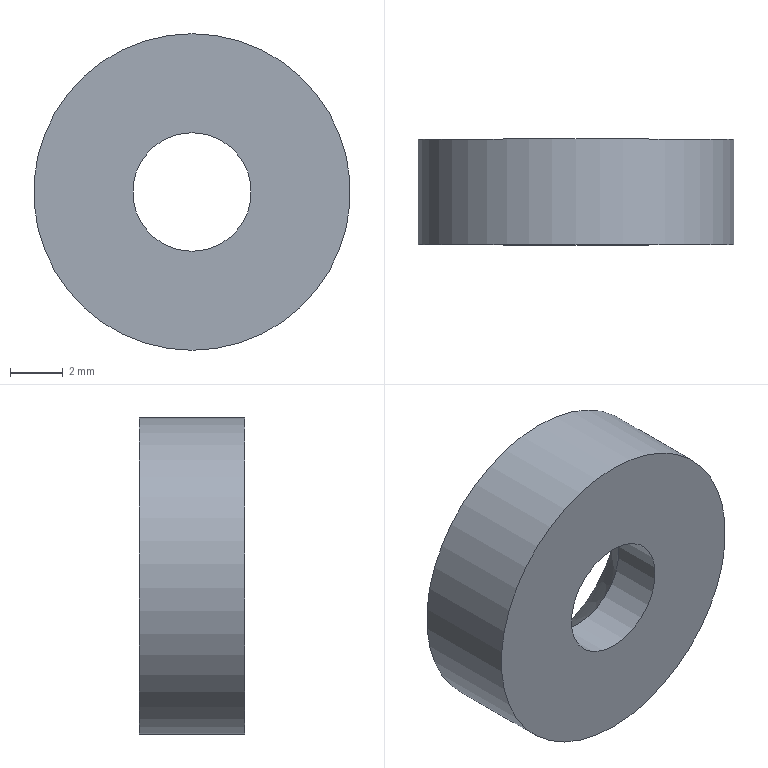Part | STEP file | Strong magnet | 1 solid | 5 faces | box 12 x 4 x 12 mm | volume 350.045 mm3 | cylinder 2 | plane 2 | cone 1 | commonest cylinder face diameters 4.5 x1 12 x1
STEP:
#1=CARTESIAN_POINT('',(0.,4.,6.));
#2=VERTEX_POINT('',#1);
#3=CARTESIAN_POINT('',(0.,4.,0.));
#4=DIRECTION('',(0.,1.,0.));
#5=DIRECTION('',(0.,0.,1.));
#6=AXIS2_PLACEMENT_3D('',#3,#4,#5);
#7=CIRCLE('',#6,6.);
#8=EDGE_CURVE('',#2,#2,#7,.T.);
#9=ORIENTED_EDGE('',*,*,#8,.F.);
#10=EDGE_LOOP('',(#9));
#11=FACE_OUTER_BOUND('',#10,.T.);
#12=CARTESIAN_POINT('',(0.,0.,6.));
#13=VERTEX_POINT('',#12);
#14=CARTESIAN_POINT('',(0.,0.,0.));
#15=DIRECTION('',(0.,1.,0.));
#16=DIRECTION('',(0.,0.,1.));
#17=AXIS2_PLACEMENT_3D('',#14,#15,#16);
#18=CIRCLE('',#17,6.);
#19=EDGE_CURVE('',#13,#13,#18,.T.);
#20=ORIENTED_EDGE('',*,*,#19,.T.);
#21=EDGE_LOOP('',(#20));
#22=FACE_OUTER_BOUND('',#21,.T.);
#23=CARTESIAN_POINT('',(0.,4.,0.));
#24=DIRECTION('',(0.,-1.,0.));
#25=DIRECTION('',(0.,0.,-1.));
#26=AXIS2_PLACEMENT_3D('',#23,#24,#25);
#27=CYLINDRICAL_SURFACE('',#26,6.);
#28=ADVANCED_FACE('',(#11,#22),#27,.T.);
#29=CARTESIAN_POINT('',(0.,4.,4.3));
#30=VERTEX_POINT('',#29);
#31=CARTESIAN_POINT('',(0.,4.,0.));
#32=DIRECTION('',(0.,1.,0.));
#33=DIRECTION('',(0.,0.,1.));
#34=AXIS2_PLACEMENT_3D('',#31,#32,#33);
#35=CIRCLE('',#34,4.3);
#36=EDGE_CURVE('',#30,#30,#35,.T.);
#37=ORIENTED_EDGE('',*,*,#36,.F.);
#38=EDGE_LOOP('',(#37));
#39=FACE_BOUND('',#38,.T.);
#40=ORIENTED_EDGE('',*,*,#8,.T.);
#41=EDGE_LOOP('',(#40));
#42=FACE_OUTER_BOUND('',#41,.T.);
#43=CARTESIAN_POINT('',(0.,4.,0.));
#44=DIRECTION('',(0.,1.,0.));
#45=DIRECTION('',(0.,0.,1.));
#46=AXIS2_PLACEMENT_3D('',#43,#44,#45);
#47=PLANE('',#46);
#48=ADVANCED_FACE('',(#39,#42),#47,.T.);
#49=CARTESIAN_POINT('',(0.,0.,2.25));
#50=VERTEX_POINT('',#49);
#51=CARTESIAN_POINT('',(0.,0.,0.));
#52=DIRECTION('',(0.,1.,0.));
#53=DIRECTION('',(0.,0.,1.));
#54=AXIS2_PLACEMENT_3D('',#51,#52,#53);
#55=CIRCLE('',#54,2.25);
#56=EDGE_CURVE('',#50,#50,#55,.T.);
#57=ORIENTED_EDGE('',*,*,#56,.T.);
#58=EDGE_LOOP('',(#57));
#59=FACE_BOUND('',#58,.T.);
#60=ORIENTED_EDGE('',*,*,#19,.F.);
#61=EDGE_LOOP('',(#60));
#62=FACE_OUTER_BOUND('',#61,.T.);
#63=CARTESIAN_POINT('',(0.,0.,0.));
#64=DIRECTION('',(0.,1.,0.));
#65=DIRECTION('',(0.,0.,1.));
#66=AXIS2_PLACEMENT_3D('',#63,#64,#65);
#67=PLANE('',#66);
#68=ADVANCED_FACE('',(#59,#62),#67,.F.);
#69=CARTESIAN_POINT('',(0.,1.95,2.25));
#70=VERTEX_POINT('',#69);
#71=CARTESIAN_POINT('',(0.,1.95,0.));
#72=DIRECTION('',(0.,1.,0.));
#73=DIRECTION('',(0.,0.,1.));
#74=AXIS2_PLACEMENT_3D('',#71,#72,#73);
#75=CIRCLE('',#74,2.25);
#76=EDGE_CURVE('',#70,#70,#75,.T.);
#77=ORIENTED_EDGE('',*,*,#76,.T.);
#78=EDGE_LOOP('',(#77));
#79=FACE_OUTER_BOUND('',#78,.T.);
#80=ORIENTED_EDGE('',*,*,#56,.F.);
#81=EDGE_LOOP('',(#80));
#82=FACE_OUTER_BOUND('',#81,.T.);
#83=CARTESIAN_POINT('',(0.,4.,0.));
#84=DIRECTION('',(0.,1.,0.));
#85=DIRECTION('',(0.,0.,1.));
#86=AXIS2_PLACEMENT_3D('',#83,#84,#85);
#87=CYLINDRICAL_SURFACE('',#86,2.25);
#88=ADVANCED_FACE('',(#79,#82),#87,.F.);
#89=ORIENTED_EDGE('',*,*,#76,.F.);
#90=EDGE_LOOP('',(#89));
#91=FACE_BOUND('',#90,.T.);
#92=ORIENTED_EDGE('',*,*,#36,.T.);
#93=EDGE_LOOP('',(#92));
#94=FACE_OUTER_BOUND('',#93,.T.);
#95=CARTESIAN_POINT('',(0.,4.,0.));
#96=DIRECTION('',(0.,1.,0.));
#97=DIRECTION('',(0.,0.,1.));
#98=AXIS2_PLACEMENT_3D('',#95,#96,#97);
#99=CONICAL_SURFACE('',#98,4.3,0.7854);
#100=ADVANCED_FACE('',(#91,#94),#99,.F.);
#101=CLOSED_SHELL('',(#28,#48,#68,#88,#100));
#102=MANIFOLD_SOLID_BREP('',#101);
#103=CARTESIAN_POINT('',(0.,0.,0.));
#104=DIRECTION('',(0.,0.,1.));
#105=DIRECTION('',(1.,0.,0.));
#106=AXIS2_PLACEMENT_3D('',#103,#104,#105);
#107=(LENGTH_UNIT()NAMED_UNIT(*)SI_UNIT(.MILLI.,.METRE.));
#108=UNCERTAINTY_MEASURE_WITH_UNIT(LENGTH_MEASURE(0.00001),#107,'','');
#109=(NAMED_UNIT(*)PLANE_ANGLE_UNIT()SI_UNIT($,.RADIAN.));
#110=(NAMED_UNIT(*)SI_UNIT($,.STERADIAN.)SOLID_ANGLE_UNIT());
#111=(GEOMETRIC_REPRESENTATION_CONTEXT(3)GLOBAL_UNCERTAINTY_ASSIGNED_CONTEXT((#108))GLOBAL_UNIT_ASSIGNED_CONTEXT((#107,#109,#110))REPRESENTATION_CONTEXT('',''));
#112=ADVANCED_BREP_SHAPE_REPRESENTATION('',(#102,#106),#111);